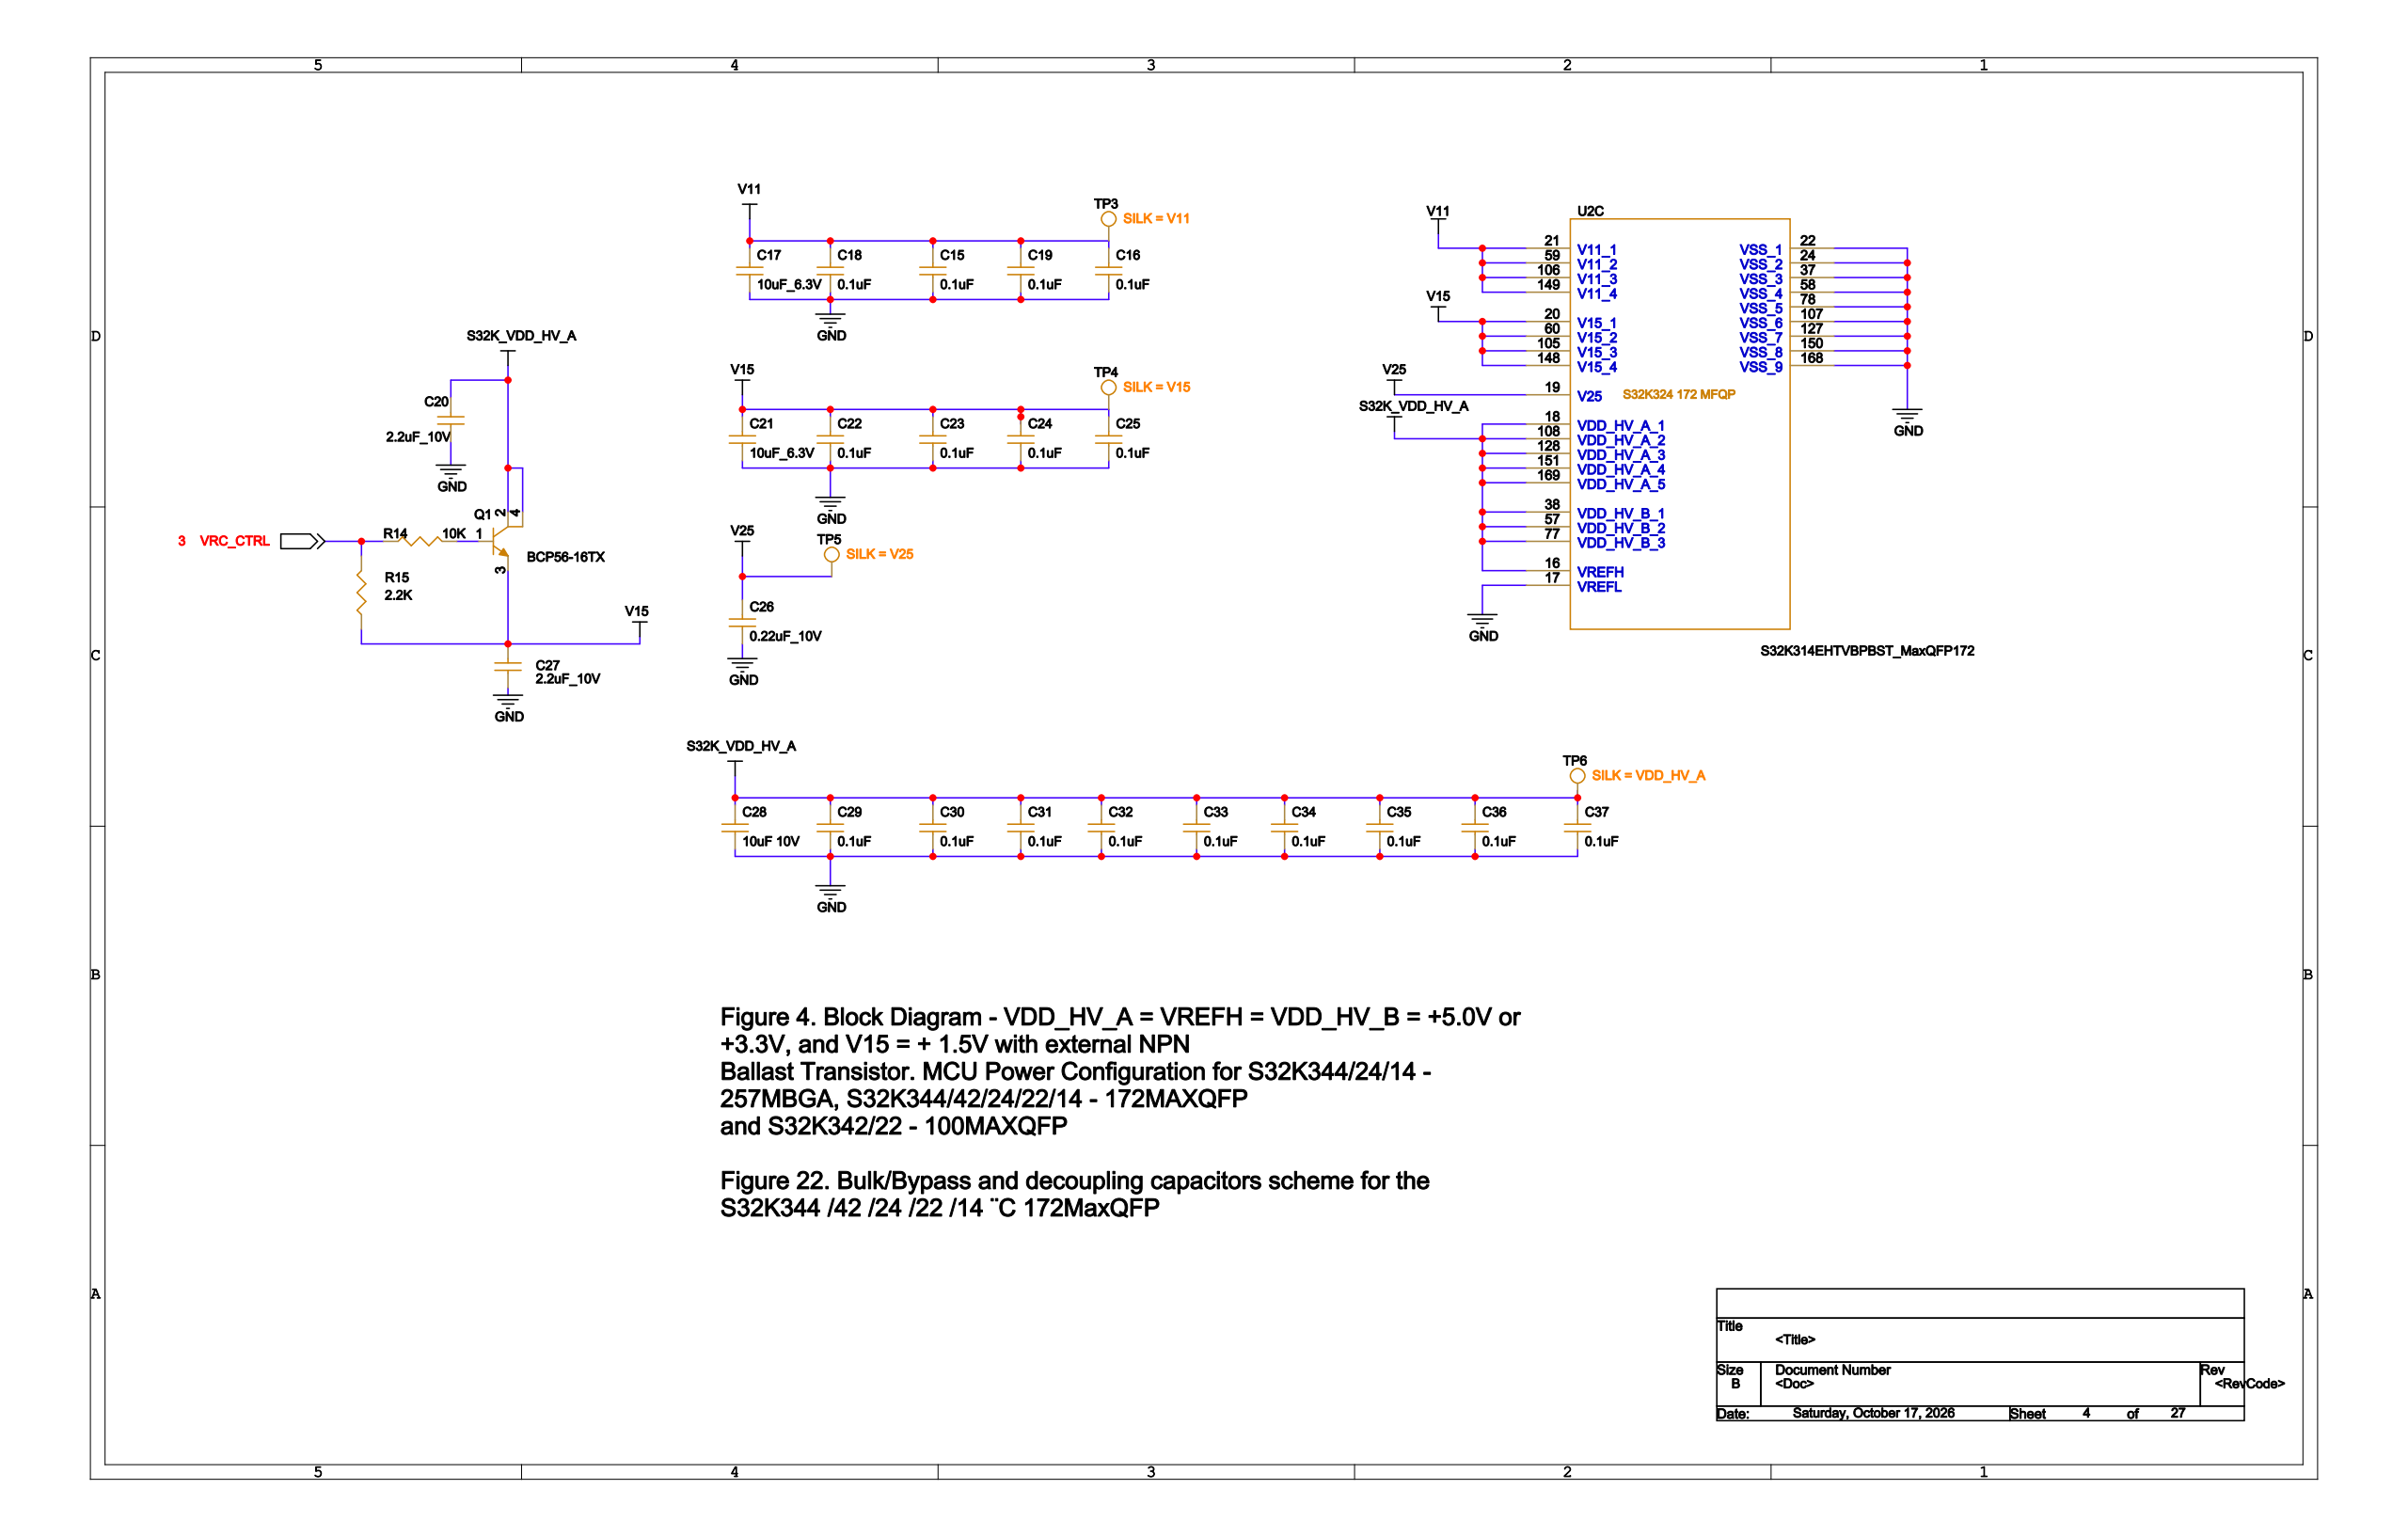Circuit board | Cadence Allegro | 477 parts | 327 nets | one sheet of the schematic
Parts on this sheet (reference | value | footprint):
C15 | 0.1uF | 0402
C16 | 0.1uF | 0402
C17 | 10uF_6.3V | 0402
C18 | 0.1uF | 0402
C19 | 0.1uF | 0402
C20 | 2.2uF_10V | 0402
C21 | 10uF_6.3V | 0402
C22 | 0.1uF | 0402
C23 | 0.1uF | 0402
C24 | 0.1uF | 0402
C25 | 0.1uF | 0402
C26 | 0.22uF_10V | 0402
C27 | 2.2uF_10V | 0402
C28 | 10uF 10V | 0603
C29 | 0.1uF | 0402
C30 | 0.1uF | 0402
C31 | 0.1uF | 0402
C32 | 0.1uF | 0402
C33 | 0.1uF | 0402
C34 | 0.1uF | 0402
C35 | 0.1uF | 0402
C36 | 0.1uF | 0402
C37 | 0.1uF | 0402
Q1 | BCP56-16TX | BCP56_SOT-223
R14 | 10K | 0402
R15 | 2.2K | 0402
TP3 | TP | S0400CI
TP4 | TP | S0400CI
TP5 | TP | S0400CI
TP6 | TP | S0400CI
U2 | S32K314EHTVBPBST_MaxQFP172 | MQFP172_0P65_16X16
Nets of these parts (net: part-pin ...):
GND: C15-1 C16-1 C17-1 C18-1 C19-1 C20-1 C21-1 C22-1 C23-1 C24-1 C25-1 C26-1 C27-1 C28-1 C29-1 C30-1 C31-1 C32-1 C33-1 C34-1 C35-1 C36-1 C37-1 U2-17 U2-22 U2-24 U2-37 U2-58 U2-78 U2-107 U2-127 U2-150 U2-168
S32K_VDD_HV_A: C20-2 C28-2 C29-2 C30-2 C31-2 C32-2 C33-2 C34-2 C35-2 C36-2 C37-2 Q1-2 Q1-4 TP6-1 U2-16 U2-18 U2-38 U2-57 U2-77 U2-108 U2-128 U2-151 U2-169
V15: C21-2 C22-2 C23-2 C24-2 C25-2 C27-2 Q1-3 R15-1 TP4-1 U2-20 U2-60 U2-105 U2-148
VRC_CTRL: R14-1 R15-2
V25: C26-2 TP5-1 U2-19
N1673456: Q1-1 R14-2
V11: C15-2 C16-2 C17-2 C18-2 C19-2 TP3-1 U2-21 U2-59 U2-106 U2-149